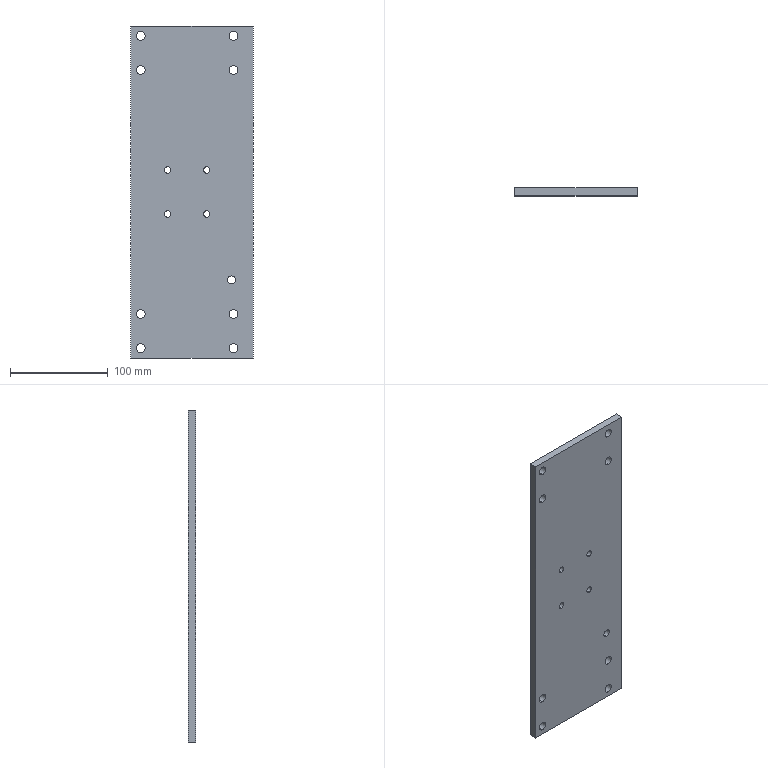Part | STEP file | X77-07101 | 1 solid | 32 faces | box 125 x 8 x 340 mm | volume 334465 mm3 | cylinder 26 | plane 6 | commonest cylinder face diameters 9 x16 6.5 x8 8 x2
STEP:
#1=CARTESIAN_POINT('',(-140.231,-59.214,-256.));
#2=VERTEX_POINT('',#1);
#3=CARTESIAN_POINT('',(-140.231,-59.214,-264.));
#4=VERTEX_POINT('',#3);
#5=CARTESIAN_POINT('',(-140.231,-59.214,-260.));
#6=DIRECTION('',(0.,-1.,0.));
#7=DIRECTION('',(1.,0.,0.));
#8=AXIS2_PLACEMENT_3D('',#5,#6,#7);
#9=CIRCLE('',#8,4.);
#10=EDGE_CURVE('',#2,#4,#9,.T.);
#11=ORIENTED_EDGE('',*,*,#10,.T.);
#12=CARTESIAN_POINT('',(-140.231,-51.214,-264.));
#13=VERTEX_POINT('',#12);
#14=CARTESIAN_POINT('',(-140.231,-51.214,-264.));
#15=DIRECTION('',(0.,1.,0.));
#16=VECTOR('',#15,1000.);
#17=LINE('',#14,#16);
#18=EDGE_CURVE('',#4,#13,#17,.T.);
#19=ORIENTED_EDGE('',*,*,#18,.T.);
#20=CARTESIAN_POINT('',(-140.231,-51.214,-256.));
#21=VERTEX_POINT('',#20);
#22=CARTESIAN_POINT('',(-140.231,-51.214,-260.));
#23=DIRECTION('',(0.,1.,0.));
#24=DIRECTION('',(0.,0.,1.));
#25=AXIS2_PLACEMENT_3D('',#22,#23,#24);
#26=CIRCLE('',#25,4.);
#27=EDGE_CURVE('',#13,#21,#26,.T.);
#28=ORIENTED_EDGE('',*,*,#27,.T.);
#29=CARTESIAN_POINT('',(-140.231,-51.214,-256.));
#30=DIRECTION('',(0.,1.,0.));
#31=VECTOR('',#30,1000.);
#32=LINE('',#29,#31);
#33=EDGE_CURVE('',#2,#21,#32,.T.);
#34=ORIENTED_EDGE('',*,*,#33,.F.);
#35=EDGE_LOOP('',(#11,#19,#28,#34));
#36=FACE_OUTER_BOUND('',#35,.T.);
#37=CARTESIAN_POINT('',(-140.231,-51.214,-260.));
#38=DIRECTION('',(0.,1.,0.));
#39=DIRECTION('',(0.,0.,1.));
#40=AXIS2_PLACEMENT_3D('',#37,#38,#39);
#41=CYLINDRICAL_SURFACE('',#40,4.);
#42=ADVANCED_FACE('',(#36),#41,.F.);
#43=CARTESIAN_POINT('',(-138.186,-51.214,-334.5));
#44=VERTEX_POINT('',#43);
#45=CARTESIAN_POINT('',(-138.186,-51.214,-325.5));
#46=VERTEX_POINT('',#45);
#47=CARTESIAN_POINT('',(-138.186,-51.214,-330.));
#48=DIRECTION('',(0.,1.,0.));
#49=DIRECTION('',(0.,0.,1.));
#50=AXIS2_PLACEMENT_3D('',#47,#48,#49);
#51=CIRCLE('',#50,4.5);
#52=EDGE_CURVE('',#44,#46,#51,.T.);
#53=ORIENTED_EDGE('',*,*,#52,.T.);
#54=CARTESIAN_POINT('',(-138.186,-59.214,-325.5));
#55=VERTEX_POINT('',#54);
#56=CARTESIAN_POINT('',(-138.186,-59.214,-325.5));
#57=DIRECTION('',(0.,-1.,0.));
#58=VECTOR('',#57,1000.);
#59=LINE('',#56,#58);
#60=EDGE_CURVE('',#46,#55,#59,.T.);
#61=ORIENTED_EDGE('',*,*,#60,.T.);
#62=CARTESIAN_POINT('',(-138.186,-59.214,-334.5));
#63=VERTEX_POINT('',#62);
#64=CARTESIAN_POINT('',(-138.186,-59.214,-330.));
#65=DIRECTION('',(0.,-1.,0.));
#66=DIRECTION('',(0.,0.,-1.));
#67=AXIS2_PLACEMENT_3D('',#64,#65,#66);
#68=CIRCLE('',#67,4.5);
#69=EDGE_CURVE('',#55,#63,#68,.T.);
#70=ORIENTED_EDGE('',*,*,#69,.T.);
#71=CARTESIAN_POINT('',(-138.186,-59.214,-334.5));
#72=DIRECTION('',(0.,-1.,0.));
#73=VECTOR('',#72,1000.);
#74=LINE('',#71,#73);
#75=EDGE_CURVE('',#44,#63,#74,.T.);
#76=ORIENTED_EDGE('',*,*,#75,.F.);
#77=EDGE_LOOP('',(#53,#61,#70,#76));
#78=FACE_OUTER_BOUND('',#77,.T.);
#79=CARTESIAN_POINT('',(-138.186,-59.214,-330.));
#80=DIRECTION('',(0.,-1.,0.));
#81=DIRECTION('',(0.,0.,-1.));
#82=AXIS2_PLACEMENT_3D('',#79,#80,#81);
#83=CYLINDRICAL_SURFACE('',#82,4.5);
#84=ADVANCED_FACE('',(#78),#83,.F.);
#85=CARTESIAN_POINT('',(-233.199,-51.214,-334.5));
#86=VERTEX_POINT('',#85);
#87=CARTESIAN_POINT('',(-233.199,-51.214,-325.5));
#88=VERTEX_POINT('',#87);
#89=CARTESIAN_POINT('',(-233.199,-51.214,-330.));
#90=DIRECTION('',(0.,1.,0.));
#91=DIRECTION('',(0.,0.,1.));
#92=AXIS2_PLACEMENT_3D('',#89,#90,#91);
#93=CIRCLE('',#92,4.5);
#94=EDGE_CURVE('',#86,#88,#93,.T.);
#95=ORIENTED_EDGE('',*,*,#94,.T.);
#96=CARTESIAN_POINT('',(-233.199,-59.214,-325.5));
#97=VERTEX_POINT('',#96);
#98=CARTESIAN_POINT('',(-233.199,-59.214,-325.5));
#99=DIRECTION('',(0.,-1.,0.));
#100=VECTOR('',#99,1000.);
#101=LINE('',#98,#100);
#102=EDGE_CURVE('',#88,#97,#101,.T.);
#103=ORIENTED_EDGE('',*,*,#102,.T.);
#104=CARTESIAN_POINT('',(-233.199,-59.214,-334.5));
#105=VERTEX_POINT('',#104);
#106=CARTESIAN_POINT('',(-233.199,-59.214,-330.));
#107=DIRECTION('',(0.,-1.,0.));
#108=DIRECTION('',(0.,0.,-1.));
#109=AXIS2_PLACEMENT_3D('',#106,#107,#108);
#110=CIRCLE('',#109,4.5);
#111=EDGE_CURVE('',#97,#105,#110,.T.);
#112=ORIENTED_EDGE('',*,*,#111,.T.);
#113=CARTESIAN_POINT('',(-233.199,-59.214,-334.5));
#114=DIRECTION('',(0.,-1.,0.));
#115=VECTOR('',#114,1000.);
#116=LINE('',#113,#115);
#117=EDGE_CURVE('',#86,#105,#116,.T.);
#118=ORIENTED_EDGE('',*,*,#117,.F.);
#119=EDGE_LOOP('',(#95,#103,#112,#118));
#120=FACE_OUTER_BOUND('',#119,.T.);
#121=CARTESIAN_POINT('',(-233.199,-59.214,-330.));
#122=DIRECTION('',(0.,-1.,0.));
#123=DIRECTION('',(0.,0.,-1.));
#124=AXIS2_PLACEMENT_3D('',#121,#122,#123);
#125=CYLINDRICAL_SURFACE('',#124,4.5);
#126=ADVANCED_FACE('',(#120),#125,.F.);
#127=CARTESIAN_POINT('',(-233.199,-51.214,-299.5));
#128=VERTEX_POINT('',#127);
#129=CARTESIAN_POINT('',(-233.199,-51.214,-290.5));
#130=VERTEX_POINT('',#129);
#131=CARTESIAN_POINT('',(-233.199,-51.214,-295.));
#132=DIRECTION('',(0.,1.,0.));
#133=DIRECTION('',(0.,0.,1.));
#134=AXIS2_PLACEMENT_3D('',#131,#132,#133);
#135=CIRCLE('',#134,4.5);
#136=EDGE_CURVE('',#128,#130,#135,.T.);
#137=ORIENTED_EDGE('',*,*,#136,.T.);
#138=CARTESIAN_POINT('',(-233.199,-59.214,-290.5));
#139=VERTEX_POINT('',#138);
#140=CARTESIAN_POINT('',(-233.199,-59.214,-290.5));
#141=DIRECTION('',(0.,-1.,0.));
#142=VECTOR('',#141,1000.);
#143=LINE('',#140,#142);
#144=EDGE_CURVE('',#130,#139,#143,.T.);
#145=ORIENTED_EDGE('',*,*,#144,.T.);
#146=CARTESIAN_POINT('',(-233.199,-59.214,-299.5));
#147=VERTEX_POINT('',#146);
#148=CARTESIAN_POINT('',(-233.199,-59.214,-295.));
#149=DIRECTION('',(0.,-1.,0.));
#150=DIRECTION('',(0.,0.,-1.));
#151=AXIS2_PLACEMENT_3D('',#148,#149,#150);
#152=CIRCLE('',#151,4.5);
#153=EDGE_CURVE('',#139,#147,#152,.T.);
#154=ORIENTED_EDGE('',*,*,#153,.T.);
#155=CARTESIAN_POINT('',(-233.199,-59.214,-299.5));
#156=DIRECTION('',(0.,-1.,0.));
#157=VECTOR('',#156,1000.);
#158=LINE('',#155,#157);
#159=EDGE_CURVE('',#128,#147,#158,.T.);
#160=ORIENTED_EDGE('',*,*,#159,.F.);
#161=EDGE_LOOP('',(#137,#145,#154,#160));
#162=FACE_OUTER_BOUND('',#161,.T.);
#163=CARTESIAN_POINT('',(-233.199,-59.214,-295.));
#164=DIRECTION('',(0.,-1.,0.));
#165=DIRECTION('',(0.,0.,-1.));
#166=AXIS2_PLACEMENT_3D('',#163,#164,#165);
#167=CYLINDRICAL_SURFACE('',#166,4.5);
#168=ADVANCED_FACE('',(#162),#167,.F.);
#169=CARTESIAN_POINT('',(-138.139,-51.214,-299.5));
#170=VERTEX_POINT('',#169);
#171=CARTESIAN_POINT('',(-138.139,-51.214,-290.5));
#172=VERTEX_POINT('',#171);
#173=CARTESIAN_POINT('',(-138.139,-51.214,-295.));
#174=DIRECTION('',(0.,1.,0.));
#175=DIRECTION('',(0.,0.,1.));
#176=AXIS2_PLACEMENT_3D('',#173,#174,#175);
#177=CIRCLE('',#176,4.5);
#178=EDGE_CURVE('',#170,#172,#177,.T.);
#179=ORIENTED_EDGE('',*,*,#178,.T.);
#180=CARTESIAN_POINT('',(-138.139,-59.214,-290.5));
#181=VERTEX_POINT('',#180);
#182=CARTESIAN_POINT('',(-138.139,-59.214,-290.5));
#183=DIRECTION('',(0.,-1.,0.));
#184=VECTOR('',#183,1000.);
#185=LINE('',#182,#184);
#186=EDGE_CURVE('',#172,#181,#185,.T.);
#187=ORIENTED_EDGE('',*,*,#186,.T.);
#188=CARTESIAN_POINT('',(-138.139,-59.214,-299.5));
#189=VERTEX_POINT('',#188);
#190=CARTESIAN_POINT('',(-138.139,-59.214,-295.));
#191=DIRECTION('',(0.,-1.,0.));
#192=DIRECTION('',(0.,0.,-1.));
#193=AXIS2_PLACEMENT_3D('',#190,#191,#192);
#194=CIRCLE('',#193,4.5);
#195=EDGE_CURVE('',#181,#189,#194,.T.);
#196=ORIENTED_EDGE('',*,*,#195,.T.);
#197=CARTESIAN_POINT('',(-138.139,-59.214,-299.5));
#198=DIRECTION('',(0.,-1.,0.));
#199=VECTOR('',#198,1000.);
#200=LINE('',#197,#199);
#201=EDGE_CURVE('',#170,#189,#200,.T.);
#202=ORIENTED_EDGE('',*,*,#201,.F.);
#203=EDGE_LOOP('',(#179,#187,#196,#202));
#204=FACE_OUTER_BOUND('',#203,.T.);
#205=CARTESIAN_POINT('',(-138.139,-59.214,-295.));
#206=DIRECTION('',(0.,-1.,0.));
#207=DIRECTION('',(0.,0.,-1.));
#208=AXIS2_PLACEMENT_3D('',#205,#206,#207);
#209=CYLINDRICAL_SURFACE('',#208,4.5);
#210=ADVANCED_FACE('',(#204),#209,.F.);
#211=CARTESIAN_POINT('',(-233.199,-51.214,-14.5));
#212=VERTEX_POINT('',#211);
#213=CARTESIAN_POINT('',(-233.199,-51.214,-5.5));
#214=VERTEX_POINT('',#213);
#215=CARTESIAN_POINT('',(-233.199,-51.214,-10.));
#216=DIRECTION('',(0.,1.,0.));
#217=DIRECTION('',(0.,0.,1.));
#218=AXIS2_PLACEMENT_3D('',#215,#216,#217);
#219=CIRCLE('',#218,4.5);
#220=EDGE_CURVE('',#212,#214,#219,.T.);
#221=ORIENTED_EDGE('',*,*,#220,.T.);
#222=CARTESIAN_POINT('',(-233.199,-59.214,-5.5));
#223=VERTEX_POINT('',#222);
#224=CARTESIAN_POINT('',(-233.199,-59.214,-5.5));
#225=DIRECTION('',(0.,-1.,0.));
#226=VECTOR('',#225,1000.);
#227=LINE('',#224,#226);
#228=EDGE_CURVE('',#214,#223,#227,.T.);
#229=ORIENTED_EDGE('',*,*,#228,.T.);
#230=CARTESIAN_POINT('',(-233.199,-59.214,-14.5));
#231=VERTEX_POINT('',#230);
#232=CARTESIAN_POINT('',(-233.199,-59.214,-10.));
#233=DIRECTION('',(0.,-1.,0.));
#234=DIRECTION('',(0.,0.,-1.));
#235=AXIS2_PLACEMENT_3D('',#232,#233,#234);
#236=CIRCLE('',#235,4.5);
#237=EDGE_CURVE('',#223,#231,#236,.T.);
#238=ORIENTED_EDGE('',*,*,#237,.T.);
#239=CARTESIAN_POINT('',(-233.199,-59.214,-14.5));
#240=DIRECTION('',(0.,-1.,0.));
#241=VECTOR('',#240,1000.);
#242=LINE('',#239,#241);
#243=EDGE_CURVE('',#212,#231,#242,.T.);
#244=ORIENTED_EDGE('',*,*,#243,.F.);
#245=EDGE_LOOP('',(#221,#229,#238,#244));
#246=FACE_OUTER_BOUND('',#245,.T.);
#247=CARTESIAN_POINT('',(-233.199,-59.214,-10.));
#248=DIRECTION('',(0.,-1.,0.));
#249=DIRECTION('',(0.,0.,-1.));
#250=AXIS2_PLACEMENT_3D('',#247,#248,#249);
#251=CYLINDRICAL_SURFACE('',#250,4.5);
#252=ADVANCED_FACE('',(#246),#251,.F.);
#253=CARTESIAN_POINT('',(-138.186,-51.214,-14.5));
#254=VERTEX_POINT('',#253);
#255=CARTESIAN_POINT('',(-138.186,-51.214,-5.5));
#256=VERTEX_POINT('',#255);
#257=CARTESIAN_POINT('',(-138.186,-51.214,-10.));
#258=DIRECTION('',(0.,1.,0.));
#259=DIRECTION('',(0.,0.,1.));
#260=AXIS2_PLACEMENT_3D('',#257,#258,#259);
#261=CIRCLE('',#260,4.5);
#262=EDGE_CURVE('',#254,#256,#261,.T.);
#263=ORIENTED_EDGE('',*,*,#262,.T.);
#264=CARTESIAN_POINT('',(-138.186,-59.214,-5.5));
#265=VERTEX_POINT('',#264);
#266=CARTESIAN_POINT('',(-138.186,-59.214,-5.5));
#267=DIRECTION('',(0.,-1.,0.));
#268=VECTOR('',#267,1000.);
#269=LINE('',#266,#268);
#270=EDGE_CURVE('',#256,#265,#269,.T.);
#271=ORIENTED_EDGE('',*,*,#270,.T.);
#272=CARTESIAN_POINT('',(-138.186,-59.214,-14.5));
#273=VERTEX_POINT('',#272);
#274=CARTESIAN_POINT('',(-138.186,-59.214,-10.));
#275=DIRECTION('',(0.,-1.,0.));
#276=DIRECTION('',(0.,0.,-1.));
#277=AXIS2_PLACEMENT_3D('',#274,#275,#276);
#278=CIRCLE('',#277,4.5);
#279=EDGE_CURVE('',#265,#273,#278,.T.);
#280=ORIENTED_EDGE('',*,*,#279,.T.);
#281=CARTESIAN_POINT('',(-138.186,-59.214,-14.5));
#282=DIRECTION('',(0.,-1.,0.));
#283=VECTOR('',#282,1000.);
#284=LINE('',#281,#283);
#285=EDGE_CURVE('',#254,#273,#284,.T.);
#286=ORIENTED_EDGE('',*,*,#285,.F.);
#287=EDGE_LOOP('',(#263,#271,#280,#286));
#288=FACE_OUTER_BOUND('',#287,.T.);
#289=CARTESIAN_POINT('',(-138.186,-59.214,-10.));
#290=DIRECTION('',(0.,-1.,0.));
#291=DIRECTION('',(0.,0.,-1.));
#292=AXIS2_PLACEMENT_3D('',#289,#290,#291);
#293=CYLINDRICAL_SURFACE('',#292,4.5);
#294=ADVANCED_FACE('',(#288),#293,.F.);
#295=CARTESIAN_POINT('',(-138.139,-51.214,-49.5));
#296=VERTEX_POINT('',#295);
#297=CARTESIAN_POINT('',(-138.139,-51.214,-40.5));
#298=VERTEX_POINT('',#297);
#299=CARTESIAN_POINT('',(-138.139,-51.214,-45.));
#300=DIRECTION('',(0.,1.,0.));
#301=DIRECTION('',(0.,0.,1.));
#302=AXIS2_PLACEMENT_3D('',#299,#300,#301);
#303=CIRCLE('',#302,4.5);
#304=EDGE_CURVE('',#296,#298,#303,.T.);
#305=ORIENTED_EDGE('',*,*,#304,.T.);
#306=CARTESIAN_POINT('',(-138.139,-59.214,-40.5));
#307=VERTEX_POINT('',#306);
#308=CARTESIAN_POINT('',(-138.139,-59.214,-40.5));
#309=DIRECTION('',(0.,-1.,0.));
#310=VECTOR('',#309,1000.);
#311=LINE('',#308,#310);
#312=EDGE_CURVE('',#298,#307,#311,.T.);
#313=ORIENTED_EDGE('',*,*,#312,.T.);
#314=CARTESIAN_POINT('',(-138.139,-59.214,-49.5));
#315=VERTEX_POINT('',#314);
#316=CARTESIAN_POINT('',(-138.139,-59.214,-45.));
#317=DIRECTION('',(0.,-1.,0.));
#318=DIRECTION('',(0.,0.,-1.));
#319=AXIS2_PLACEMENT_3D('',#316,#317,#318);
#320=CIRCLE('',#319,4.5);
#321=EDGE_CURVE('',#307,#315,#320,.T.);
#322=ORIENTED_EDGE('',*,*,#321,.T.);
#323=CARTESIAN_POINT('',(-138.139,-59.214,-49.5));
#324=DIRECTION('',(0.,-1.,0.));
#325=VECTOR('',#324,1000.);
#326=LINE('',#323,#325);
#327=EDGE_CURVE('',#296,#315,#326,.T.);
#328=ORIENTED_EDGE('',*,*,#327,.F.);
#329=EDGE_LOOP('',(#305,#313,#322,#328));
#330=FACE_OUTER_BOUND('',#329,.T.);
#331=CARTESIAN_POINT('',(-138.139,-59.214,-45.));
#332=DIRECTION('',(0.,-1.,0.));
#333=DIRECTION('',(0.,0.,-1.));
#334=AXIS2_PLACEMENT_3D('',#331,#332,#333);
#335=CYLINDRICAL_SURFACE('',#334,4.5);
#336=ADVANCED_FACE('',(#330),#335,.F.);
#337=CARTESIAN_POINT('',(-233.199,-51.214,-49.5));
#338=VERTEX_POINT('',#337);
#339=CARTESIAN_POINT('',(-233.199,-51.214,-40.5));
#340=VERTEX_POINT('',#339);
#341=CARTESIAN_POINT('',(-233.199,-51.214,-45.));
#342=DIRECTION('',(0.,1.,0.));
#343=DIRECTION('',(0.,0.,1.));
#344=AXIS2_PLACEMENT_3D('',#341,#342,#343);
#345=CIRCLE('',#344,4.5);
#346=EDGE_CURVE('',#338,#340,#345,.T.);
#347=ORIENTED_EDGE('',*,*,#346,.T.);
#348=CARTESIAN_POINT('',(-233.199,-59.214,-40.5));
#349=VERTEX_POINT('',#348);
#350=CARTESIAN_POINT('',(-233.199,-59.214,-40.5));
#351=DIRECTION('',(0.,-1.,0.));
#352=VECTOR('',#351,1000.);
#353=LINE('',#350,#352);
#354=EDGE_CURVE('',#340,#349,#353,.T.);
#355=ORIENTED_EDGE('',*,*,#354,.T.);
#356=CARTESIAN_POINT('',(-233.199,-59.214,-49.5));
#357=VERTEX_POINT('',#356);
#358=CARTESIAN_POINT('',(-233.199,-59.214,-45.));
#359=DIRECTION('',(0.,-1.,0.));
#360=DIRECTION('',(0.,0.,-1.));
#361=AXIS2_PLACEMENT_3D('',#358,#359,#360);
#362=CIRCLE('',#361,4.5);
#363=EDGE_CURVE('',#349,#357,#362,.T.);
#364=ORIENTED_EDGE('',*,*,#363,.T.);
#365=CARTESIAN_POINT('',(-233.199,-59.214,-49.5));
#366=DIRECTION('',(0.,-1.,0.));
#367=VECTOR('',#366,1000.);
#368=LINE('',#365,#367);
#369=EDGE_CURVE('',#338,#357,#368,.T.);
#370=ORIENTED_EDGE('',*,*,#369,.F.);
#371=EDGE_LOOP('',(#347,#355,#364,#370));
#372=FACE_OUTER_BOUND('',#371,.T.);
#373=CARTESIAN_POINT('',(-233.199,-59.214,-45.));
#374=DIRECTION('',(0.,-1.,0.));
#375=DIRECTION('',(0.,0.,-1.));
#376=AXIS2_PLACEMENT_3D('',#373,#374,#375);
#377=CYLINDRICAL_SURFACE('',#376,4.5);
#378=ADVANCED_FACE('',(#372),#377,.F.);
#379=CARTESIAN_POINT('',(-205.699,-51.214,-195.75));
#380=VERTEX_POINT('',#379);
#381=CARTESIAN_POINT('',(-205.699,-51.214,-189.25));
#382=VERTEX_POINT('',#381);
#383=CARTESIAN_POINT('',(-205.699,-51.214,-192.5));
#384=DIRECTION('',(0.,1.,0.));
#385=DIRECTION('',(0.,0.,1.));
#386=AXIS2_PLACEMENT_3D('',#383,#384,#385);
#387=CIRCLE('',#386,3.25);
#388=EDGE_CURVE('',#380,#382,#387,.T.);
#389=ORIENTED_EDGE('',*,*,#388,.T.);
#390=CARTESIAN_POINT('',(-205.699,-59.214,-189.25));
#391=VERTEX_POINT('',#390);
#392=CARTESIAN_POINT('',(-205.699,-59.214,-189.25));
#393=DIRECTION('',(0.,-1.,0.));
#394=VECTOR('',#393,1000.);
#395=LINE('',#392,#394);
#396=EDGE_CURVE('',#382,#391,#395,.T.);
#397=ORIENTED_EDGE('',*,*,#396,.T.);
#398=CARTESIAN_POINT('',(-205.699,-59.214,-195.75));
#399=VERTEX_POINT('',#398);
#400=CARTESIAN_POINT('',(-205.699,-59.214,-192.5));
#401=DIRECTION('',(0.,-1.,0.));
#402=DIRECTION('',(0.,0.,-1.));
#403=AXIS2_PLACEMENT_3D('',#400,#401,#402);
#404=CIRCLE('',#403,3.25);
#405=EDGE_CURVE('',#391,#399,#404,.T.);
#406=ORIENTED_EDGE('',*,*,#405,.T.);
#407=CARTESIAN_POINT('',(-205.699,-59.214,-195.75));
#408=DIRECTION('',(0.,-1.,0.));
#409=VECTOR('',#408,1000.);
#410=LINE('',#407,#409);
#411=EDGE_CURVE('',#380,#399,#410,.T.);
#412=ORIENTED_EDGE('',*,*,#411,.F.);
#413=EDGE_LOOP('',(#389,#397,#406,#412));
#414=FACE_OUTER_BOUND('',#413,.T.);
#415=CARTESIAN_POINT('',(-205.699,-59.214,-192.5));
#416=DIRECTION('',(0.,-1.,0.));
#417=DIRECTION('',(0.,0.,-1.));
#418=AXIS2_PLACEMENT_3D('',#415,#416,#417);
#419=CYLINDRICAL_SURFACE('',#418,3.25);
#420=ADVANCED_FACE('',(#414),#419,.F.);
#421=CARTESIAN_POINT('',(-205.699,-51.214,-150.75));
#422=VERTEX_POINT('',#421);
#423=CARTESIAN_POINT('',(-205.699,-51.214,-144.25));
#424=VERTEX_POINT('',#423);
#425=CARTESIAN_POINT('',(-205.699,-51.214,-147.5));
#426=DIRECTION('',(0.,1.,0.));
#427=DIRECTION('',(0.,0.,1.));
#428=AXIS2_PLACEMENT_3D('',#425,#426,#427);
#429=CIRCLE('',#428,3.25);
#430=EDGE_CURVE('',#422,#424,#429,.T.);
#431=ORIENTED_EDGE('',*,*,#430,.T.);
#432=CARTESIAN_POINT('',(-205.699,-59.214,-144.25));
#433=VERTEX_POINT('',#432);
#434=CARTESIAN_POINT('',(-205.699,-59.214,-144.25));
#435=DIRECTION('',(0.,-1.,0.));
#436=VECTOR('',#435,1000.);
#437=LINE('',#434,#436);
#438=EDGE_CURVE('',#424,#433,#437,.T.);
#439=ORIENTED_EDGE('',*,*,#438,.T.);
#440=CARTESIAN_POINT('',(-205.699,-59.214,-150.75));
#441=VERTEX_POINT('',#440);
#442=CARTESIAN_POINT('',(-205.699,-59.214,-147.5));
#443=DIRECTION('',(0.,-1.,0.));
#444=DIRECTION('',(0.,0.,-1.));
#445=AXIS2_PLACEMENT_3D('',#442,#443,#444);
#446=CIRCLE('',#445,3.25);
#447=EDGE_CURVE('',#433,#441,#446,.T.);
#448=ORIENTED_EDGE('',*,*,#447,.T.);
#449=CARTESIAN_POINT('',(-205.699,-59.214,-150.75));
#450=DIRECTION('',(0.,-1.,0.));
#451=VECTOR('',#450,1000.);
#452=LINE('',#449,#451);
#453=EDGE_CURVE('',#422,#441,#452,.T.);
#454=ORIENTED_EDGE('',*,*,#453,.F.);
#455=EDGE_LOOP('',(#431,#439,#448,#454));
#456=FACE_OUTER_BOUND('',#455,.T.);
#457=CARTESIAN_POINT('',(-205.699,-59.214,-147.5));
#458=DIRECTION('',(0.,-1.,0.));
#459=DIRECTION('',(0.,0.,-1.));
#460=AXIS2_PLACEMENT_3D('',#457,#458,#459);
#461=CYLINDRICAL_SURFACE('',#460,3.25);
#462=ADVANCED_FACE('',(#456),#461,.F.);
#463=CARTESIAN_POINT('',(-165.699,-51.214,-195.75));
#464=VERTEX_POINT('',#463);
#465=CARTESIAN_POINT('',(-165.699,-51.214,-189.25));
#466=VERTEX_POINT('',#465);
#467=CARTESIAN_POINT('',(-165.699,-51.214,-192.5));
#468=DIRECTION('',(0.,1.,0.));
#469=DIRECTION('',(0.,0.,1.));
#470=AXIS2_PLACEMENT_3D('',#467,#468,#469);
#471=CIRCLE('',#470,3.25);
#472=EDGE_CURVE('',#464,#466,#471,.T.);
#473=ORIENTED_EDGE('',*,*,#472,.T.);
#474=CARTESIAN_POINT('',(-165.699,-59.214,-189.25));
#475=VERTEX_POINT('',#474);
#476=CARTESIAN_POINT('',(-165.699,-59.214,-189.25));
#477=DIRECTION('',(0.,-1.,0.));
#478=VECTOR('',#477,1000.);
#479=LINE('',#476,#478);
#480=EDGE_CURVE('',#466,#475,#479,.T.);
#481=ORIENTED_EDGE('',*,*,#480,.T.);
#482=CARTESIAN_POINT('',(-165.699,-59.214,-195.75));
#483=VERTEX_POINT('',#482);
#484=CARTESIAN_POINT('',(-165.699,-59.214,-192.5));
#485=DIRECTION('',(0.,-1.,0.));
#486=DIRECTION('',(0.,0.,-1.));
#487=AXIS2_PLACEMENT_3D('',#484,#485,#486);
#488=CIRCLE('',#487,3.25);
#489=EDGE_CURVE('',#475,#483,#488,.T.);
#490=ORIENTED_EDGE('',*,*,#489,.T.);
#491=CARTESIAN_POINT('',(-165.699,-59.214,-195.75));
#492=DIRECTION('',(0.,-1.,0.));
#493=VECTOR('',#492,1000.);
#494=LINE('',#491,#493);
#495=EDGE_CURVE('',#464,#483,#494,.T.);
#496=ORIENTED_EDGE('',*,*,#495,.F.);
#497=EDGE_LOOP('',(#473,#481,#490,#496));
#498=FACE_OUTER_BOUND('',#497,.T.);
#499=CARTESIAN_POINT('',(-165.699,-59.214,-192.5));
#500=DIRECTION('',(0.,-1.,0.));
#501=DIRECTION('',(0.,0.,-1.));
#502=AXIS2_PLACEMENT_3D('',#499,#500,#501);
#503=CYLINDRICAL_SURFACE('',#502,3.25);
#504=ADVANCED_FACE('',(#498),#503,.F.);
#505=CARTESIAN_POINT('',(-165.699,-51.214,-150.75));
#506=VERTEX_POINT('',#505);
#507=CARTESIAN_POINT('',(-165.699,-51.214,-144.25));
#508=VERTEX_POINT('',#507);
#509=CARTESIAN_POINT('',(-165.699,-51.214,-147.5));
#510=DIRECTION('',(0.,1.,0.));
#511=DIRECTION('',(0.,0.,1.));
#512=AXIS2_PLACEMENT_3D('',#509,#510,#511);
#513=CIRCLE('',#512,3.25);
#514=EDGE_CURVE('',#506,#508,#513,.T.);
#515=ORIENTED_EDGE('',*,*,#514,.T.);
#516=CARTESIAN_POINT('',(-165.699,-59.214,-144.25));
#517=VERTEX_POINT('',#516);
#518=CARTESIAN_POINT('',(-165.699,-59.214,-144.25));
#519=DIRECTION('',(0.,-1.,0.));
#520=VECTOR('',#519,1000.);
#521=LINE('',#518,#520);
#522=EDGE_CURVE('',#508,#517,#521,.T.);
#523=ORIENTED_EDGE('',*,*,#522,.T.);
#524=CARTESIAN_POINT('',(-165.699,-59.214,-150.75));
#525=VERTEX_POINT('',#524);
#526=CARTESIAN_POINT('',(-165.699,-59.214,-147.5));
#527=DIRECTION('',(0.,-1.,0.));
#528=DIRECTION('',(0.,0.,-1.));
#529=AXIS2_PLACEMENT_3D('',#526,#527,#528);
#530=CIRCLE('',#529,3.25);
#531=EDGE_CURVE('',#517,#525,#530,.T.);
#532=ORIENTED_EDGE('',*,*,#531,.T.);
#533=CARTESIAN_POINT('',(-165.699,-59.214,-150.75));
#534=DIRECTION('',(0.,-1.,0.));
#535=VECTOR('',#534,1000.);
#536=LINE('',#533,#535);
#537=EDGE_CURVE('',#506,#525,#536,.T.);
#538=ORIENTED_EDGE('',*,*,#537,.F.);
#539=EDGE_LOOP('',(#515,#523,#532,#538));
#540=FACE_OUTER_BOUND('',#539,.T.);
#541=CARTESIAN_POINT('',(-165.699,-59.214,-147.5));
#542=DIRECTION('',(0.,-1.,0.));
#543=DIRECTION('',(0.,0.,-1.));
#544=AXIS2_PLACEMENT_3D('',#541,#542,#543);
#545=CYLINDRICAL_SURFACE('',#544,3.25);
#546=ADVANCED_FACE('',(#540),#545,.F.);
#547=CARTESIAN_POINT('',(-243.199,-51.214,0.));
#548=VERTEX_POINT('',#547);
#549=CARTESIAN_POINT('',(-243.199,-59.214,0.));
#550=VERTEX_POINT('',#549);
#551=CARTESIAN_POINT('',(-243.199,-51.214,0.));
#552=DIRECTION('',(0.,-1.,0.));
#553=VECTOR('',#552,1000.);
#554=LINE('',#551,#553);
#555=EDGE_CURVE('',#548,#550,#554,.T.);
#556=ORIENTED_EDGE('',*,*,#555,.F.);
#557=CARTESIAN_POINT('',(-243.199,-51.214,-340.));
#558=VERTEX_POINT('',#557);
#559=CARTESIAN_POINT('',(-243.199,-51.214,-340.));
#560=DIRECTION('',(0.,0.,1.));
#561=VECTOR('',#560,1000.);
#562=LINE('',#559,#561);
#563=EDGE_CURVE('',#558,#548,#562,.T.);
#564=ORIENTED_EDGE('',*,*,#563,.F.);
#565=CARTESIAN_POINT('',(-243.199,-59.214,-340.));
#566=VERTEX_POINT('',#565);
#567=CARTESIAN_POINT('',(-243.199,-51.214,-340.));
#568=DIRECTION('',(0.,-1.,0.));
#569=VECTOR('',#568,1000.);
#570=LINE('',#567,#569);
#571=EDGE_CURVE('',#558,#566,#570,.T.);
#572=ORIENTED_EDGE('',*,*,#571,.T.);
#573=CARTESIAN_POINT('',(-243.199,-59.214,-340.));
#574=DIRECTION('',(0.,0.,1.));
#575=VECTOR('',#574,1000.);
#576=LINE('',#573,#575);
#577=EDGE_CURVE('',#566,#550,#576,.T.);
#578=ORIENTED_EDGE('',*,*,#577,.T.);
#579=EDGE_LOOP('',(#556,#564,#572,#578));
#580=FACE_OUTER_BOUND('',#579,.T.);
#581=CARTESIAN_POINT('',(-243.199,-51.214,-340.));
#582=DIRECTION('',(-1.,0.,0.));
#583=DIRECTION('',(0.,0.,1.));
#584=AXIS2_PLACEMENT_3D('',#581,#582,#583);
#585=PLANE('',#584);
#586=ADVANCED_FACE('',(#580),#585,.T.);
#587=CARTESIAN_POINT('',(-140.231,-51.214,-260.));
#588=DIRECTION('',(0.,1.,0.));
#589=DIRECTION('',(0.,0.,1.));
#590=AXIS2_PLACEMENT_3D('',#587,#588,#589);
#591=CIRCLE('',#590,4.);
#592=EDGE_CURVE('',#21,#13,#591,.T.);
#593=ORIENTED_EDGE('',*,*,#592,.F.);
#594=ORIENTED_EDGE('',*,*,#27,.F.);
#595=EDGE_LOOP('',(#593,#594));
#596=FACE_BOUND('',#595,.T.);
#597=ORIENTED_EDGE('',*,*,#52,.F.);
#598=CARTESIAN_POINT('',(-138.186,-51.214,-330.));
#599=DIRECTION('',(0.,1.,0.));
#600=DIRECTION('',(0.,0.,1.));
#601=AXIS2_PLACEMENT_3D('',#598,#599,#600);
#602=CIRCLE('',#601,4.5);
#603=EDGE_CURVE('',#46,#44,#602,.T.);
#604=ORIENTED_EDGE('',*,*,#603,.F.);
#605=EDGE_LOOP('',(#597,#604));
#606=FACE_BOUND('',#605,.T.);
#607=ORIENTED_EDGE('',*,*,#94,.F.);
#608=CARTESIAN_POINT('',(-233.199,-51.214,-330.));
#609=DIRECTION('',(0.,1.,0.));
#610=DIRECTION('',(0.,0.,1.));
#611=AXIS2_PLACEMENT_3D('',#608,#609,#610);
#612=CIRCLE('',#611,4.5);
#613=EDGE_CURVE('',#88,#86,#612,.T.);
#614=ORIENTED_EDGE('',*,*,#613,.F.);
#615=EDGE_LOOP('',(#607,#614));
#616=FACE_BOUND('',#615,.T.);
#617=ORIENTED_EDGE('',*,*,#136,.F.);
#618=CARTESIAN_POINT('',(-233.199,-51.214,-295.));
#619=DIRECTION('',(0.,1.,0.));
#620=DIRECTION('',(0.,0.,1.));
#621=AXIS2_PLACEMENT_3D('',#618,#619,#620);
#622=CIRCLE('',#621,4.5);
#623=EDGE_CURVE('',#130,#128,#622,.T.);
#624=ORIENTED_EDGE('',*,*,#623,.F.);
#625=EDGE_LOOP('',(#617,#624));
#626=FACE_BOUND('',#625,.T.);
#627=ORIENTED_EDGE('',*,*,#178,.F.);
#628=CARTESIAN_POINT('',(-138.139,-51.214,-295.));
#629=DIRECTION('',(0.,1.,0.));
#630=DIRECTION('',(0.,0.,1.));
#631=AXIS2_PLACEMENT_3D('',#628,#629,#630);
#632=CIRCLE('',#631,4.5);
#633=EDGE_CURVE('',#172,#170,#632,.T.);
#634=ORIENTED_EDGE('',*,*,#633,.F.);
#635=EDGE_LOOP('',(#627,#634));
#636=FACE_BOUND('',#635,.T.);
#637=ORIENTED_EDGE('',*,*,#220,.F.);
#638=CARTESIAN_POINT('',(-233.199,-51.214,-10.));
#639=DIRECTION('',(0.,1.,0.));
#640=DIRECTION('',(0.,0.,1.));
#641=AXIS2_PLACEMENT_3D('',#638,#639,#640);
#642=CIRCLE('',#641,4.5);
#643=EDGE_CURVE('',#214,#212,#642,.T.);
#644=ORIENTED_EDGE('',*,*,#643,.F.);
#645=EDGE_LOOP('',(#637,#644));
#646=FACE_BOUND('',#645,.T.);
#647=ORIENTED_EDGE('',*,*,#262,.F.);
#648=CARTESIAN_POINT('',(-138.186,-51.214,-10.));
#649=DIRECTION('',(0.,1.,0.));
#650=DIRECTION('',(0.,0.,1.));
#651=AXIS2_PLACEMENT_3D('',#648,#649,#650);
#652=CIRCLE('',#651,4.5);
#653=EDGE_CURVE('',#256,#254,#652,.T.);
#654=ORIENTED_EDGE('',*,*,#653,.F.);
#655=EDGE_LOOP('',(#647,#654));
#656=FACE_BOUND('',#655,.T.);
#657=ORIENTED_EDGE('',*,*,#304,.F.);
#658=CARTESIAN_POINT('',(-138.139,-51.214,-45.));
#659=DIRECTION('',(0.,1.,0.));
#660=DIRECTION('',(0.,0.,1.));
#661=AXIS2_PLACEMENT_3D('',#658,#659,#660);
#662=CIRCLE('',#661,4.5);
#663=EDGE_CURVE('',#298,#296,#662,.T.);
#664=ORIENTED_EDGE('',*,*,#663,.F.);
#665=EDGE_LOOP('',(#657,#664));
#666=FACE_BOUND('',#665,.T.);
#667=ORIENTED_EDGE('',*,*,#346,.F.);
#668=CARTESIAN_POINT('',(-233.199,-51.214,-45.));
#669=DIRECTION('',(0.,1.,0.));
#670=DIRECTION('',(0.,0.,1.));
#671=AXIS2_PLACEMENT_3D('',#668,#669,#670);
#672=CIRCLE('',#671,4.5);
#673=EDGE_CURVE('',#340,#338,#672,.T.);
#674=ORIENTED_EDGE('',*,*,#673,.F.);
#675=EDGE_LOOP('',(#667,#674));
#676=FACE_BOUND('',#675,.T.);
#677=ORIENTED_EDGE('',*,*,#388,.F.);
#678=CARTESIAN_POINT('',(-205.699,-51.214,-192.5));
#679=DIRECTION('',(0.,1.,0.));
#680=DIRECTION('',(0.,0.,1.));
#681=AXIS2_PLACEMENT_3D('',#678,#679,#680);
#682=CIRCLE('',#681,3.25);
#683=EDGE_CURVE('',#382,#380,#682,.T.);
#684=ORIENTED_EDGE('',*,*,#683,.F.);
#685=EDGE_LOOP('',(#677,#684));
#686=FACE_BOUND('',#685,.T.);
#687=ORIENTED_EDGE('',*,*,#430,.F.);
#688=CARTESIAN_POINT('',(-205.699,-51.214,-147.5));
#689=DIRECTION('',(0.,1.,0.));
#690=DIRECTION('',(0.,0.,1.));
#691=AXIS2_PLACEMENT_3D('',#688,#689,#690);
#692=CIRCLE('',#691,3.25);
#693=EDGE_CURVE('',#424,#422,#692,.T.);
#694=ORIENTED_EDGE('',*,*,#693,.F.);
#695=EDGE_LOOP('',(#687,#694));
#696=FACE_BOUND('',#695,.T.);
#697=ORIENTED_EDGE('',*,*,#472,.F.);
#698=CARTESIAN_POINT('',(-165.699,-51.214,-192.5));
#699=DIRECTION('',(0.,1.,0.));
#700=DIRECTION('',(0.,0.,1.));
#701=AXIS2_PLACEMENT_3D('',#698,#699,#700);
#702=CIRCLE('',#701,3.25);
#703=EDGE_CURVE('',#466,#464,#702,.T.);
#704=ORIENTED_EDGE('',*,*,#703,.F.);
#705=EDGE_LOOP('',(#697,#704));
#706=FACE_BOUND('',#705,.T.);
#707=ORIENTED_EDGE('',*,*,#514,.F.);
#708=CARTESIAN_POINT('',(-165.699,-51.214,-147.5));
#709=DIRECTION('',(0.,1.,0.));
#710=DIRECTION('',(0.,0.,1.));
#711=AXIS2_PLACEMENT_3D('',#708,#709,#710);
#712=CIRCLE('',#711,3.25);
#713=EDGE_CURVE('',#508,#506,#712,.T.);
#714=ORIENTED_EDGE('',*,*,#713,.F.);
#715=EDGE_LOOP('',(#707,#714));
#716=FACE_BOUND('',#715,.T.);
#717=CARTESIAN_POINT('',(-118.199,-51.214,0.));
#718=VERTEX_POINT('',#717);
#719=CARTESIAN_POINT('',(-243.199,-51.214,0.));
#720=DIRECTION('',(-1.,0.,0.));
#721=VECTOR('',#720,1000.);
#722=LINE('',#719,#721);
#723=EDGE_CURVE('',#718,#548,#722,.T.);
#724=ORIENTED_EDGE('',*,*,#723,.F.);
#725=CARTESIAN_POINT('',(-118.199,-51.214,-340.));
#726=VERTEX_POINT('',#725);
#727=CARTESIAN_POINT('',(-118.199,-51.214,-340.));
#728=DIRECTION('',(0.,0.,1.));
#729=VECTOR('',#728,1000.);
#730=LINE('',#727,#729);
#731=EDGE_CURVE('',#726,#718,#730,.T.);
#732=ORIENTED_EDGE('',*,*,#731,.F.);
#733=CARTESIAN_POINT('',(-243.199,-51.214,-340.));
#734=DIRECTION('',(-1.,0.,0.));
#735=VECTOR('',#734,1000.);
#736=LINE('',#733,#735);
#737=EDGE_CURVE('',#726,#558,#736,.T.);
#738=ORIENTED_EDGE('',*,*,#737,.T.);
#739=ORIENTED_EDGE('',*,*,#563,.T.);
#740=EDGE_LOOP('',(#724,#732,#738,#739));
#741=FACE_OUTER_BOUND('',#740,.T.);
#742=CARTESIAN_POINT('',(-243.199,-51.214,-340.));
#743=DIRECTION('',(0.,1.,0.));
#744=DIRECTION('',(0.,0.,1.));
#745=AXIS2_PLACEMENT_3D('',#742,#743,#744);
#746=PLANE('',#745);
#747=ADVANCED_FACE('',(#596,#606,#616,#626,#636,#646,#656,#666,#676,#686,#696,#706,#716,#741),#746,.T.);
#748=CARTESIAN_POINT('',(-118.199,-59.214,0.));
#749=VERTEX_POINT('',#748);
#750=CARTESIAN_POINT('',(-118.199,-51.214,0.));
#751=DIRECTION('',(0.,1.,0.));
#752=VECTOR('',#751,1000.);
#753=LINE('',#750,#752);
#754=EDGE_CURVE('',#749,#718,#753,.T.);
#755=ORIENTED_EDGE('',*,*,#754,.F.);
#756=CARTESIAN_POINT('',(-118.199,-59.214,-340.));
#757=VERTEX_POINT('',#756);
#758=CARTESIAN_POINT('',(-118.199,-59.214,-340.));
#759=DIRECTION('',(0.,0.,1.));
#760=VECTOR('',#759,1000.);
#761=LINE('',#758,#760);
#762=EDGE_CURVE('',#757,#749,#761,.T.);
#763=ORIENTED_EDGE('',*,*,#762,.F.);
#764=CARTESIAN_POINT('',(-118.199,-51.214,-340.));
#765=DIRECTION('',(0.,1.,0.));
#766=VECTOR('',#765,1000.);
#767=LINE('',#764,#766);
#768=EDGE_CURVE('',#757,#726,#767,.T.);
#769=ORIENTED_EDGE('',*,*,#768,.T.);
#770=ORIENTED_EDGE('',*,*,#731,.T.);
#771=EDGE_LOOP('',(#755,#763,#769,#770));
#772=FACE_OUTER_BOUND('',#771,.T.);
#773=CARTESIAN_POINT('',(-118.199,-51.214,-340.));
#774=DIRECTION('',(1.,0.,0.));
#775=DIRECTION('',(0.,0.,-1.));
#776=AXIS2_PLACEMENT_3D('',#773,#774,#775);
#777=PLANE('',#776);
#778=ADVANCED_FACE('',(#772),#777,.T.);
#779=ORIENTED_EDGE('',*,*,#10,.F.);
#780=CARTESIAN_POINT('',(-140.231,-59.214,-260.));
#781=DIRECTION('',(0.,-1.,0.));
#782=DIRECTION('',(1.,0.,0.));
#783=AXIS2_PLACEMENT_3D('',#780,#781,#782);
#784=CIRCLE('',#783,4.);
#785=EDGE_CURVE('',#4,#2,#784,.T.);
#786=ORIENTED_EDGE('',*,*,#785,.F.);
#787=EDGE_LOOP('',(#779,#786));
#788=FACE_BOUND('',#787,.T.);
#789=CARTESIAN_POINT('',(-138.186,-59.214,-330.));
#790=DIRECTION('',(0.,-1.,0.));
#791=DIRECTION('',(0.,0.,-1.));
#792=AXIS2_PLACEMENT_3D('',#789,#790,#791);
#793=CIRCLE('',#792,4.5);
#794=EDGE_CURVE('',#63,#55,#793,.T.);
#795=ORIENTED_EDGE('',*,*,#794,.F.);
#796=ORIENTED_EDGE('',*,*,#69,.F.);
#797=EDGE_LOOP('',(#795,#796));
#798=FACE_BOUND('',#797,.T.);
#799=CARTESIAN_POINT('',(-233.199,-59.214,-330.));
#800=DIRECTION('',(0.,-1.,0.));
#801=DIRECTION('',(0.,0.,-1.));
#802=AXIS2_PLACEMENT_3D('',#799,#800,#801);
#803=CIRCLE('',#802,4.5);
#804=EDGE_CURVE('',#105,#97,#803,.T.);
#805=ORIENTED_EDGE('',*,*,#804,.F.);
#806=ORIENTED_EDGE('',*,*,#111,.F.);
#807=EDGE_LOOP('',(#805,#806));
#808=FACE_BOUND('',#807,.T.);
#809=CARTESIAN_POINT('',(-233.199,-59.214,-295.));
#810=DIRECTION('',(0.,-1.,0.));
#811=DIRECTION('',(0.,0.,-1.));
#812=AXIS2_PLACEMENT_3D('',#809,#810,#811);
#813=CIRCLE('',#812,4.5);
#814=EDGE_CURVE('',#147,#139,#813,.T.);
#815=ORIENTED_EDGE('',*,*,#814,.F.);
#816=ORIENTED_EDGE('',*,*,#153,.F.);
#817=EDGE_LOOP('',(#815,#816));
#818=FACE_BOUND('',#817,.T.);
#819=CARTESIAN_POINT('',(-138.139,-59.214,-295.));
#820=DIRECTION('',(0.,-1.,0.));
#821=DIRECTION('',(0.,0.,-1.));
#822=AXIS2_PLACEMENT_3D('',#819,#820,#821);
#823=CIRCLE('',#822,4.5);
#824=EDGE_CURVE('',#189,#181,#823,.T.);
#825=ORIENTED_EDGE('',*,*,#824,.F.);
#826=ORIENTED_EDGE('',*,*,#195,.F.);
#827=EDGE_LOOP('',(#825,#826));
#828=FACE_BOUND('',#827,.T.);
#829=CARTESIAN_POINT('',(-233.199,-59.214,-10.));
#830=DIRECTION('',(0.,-1.,0.));
#831=DIRECTION('',(0.,0.,-1.));
#832=AXIS2_PLACEMENT_3D('',#829,#830,#831);
#833=CIRCLE('',#832,4.5);
#834=EDGE_CURVE('',#231,#223,#833,.T.);
#835=ORIENTED_EDGE('',*,*,#834,.F.);
#836=ORIENTED_EDGE('',*,*,#237,.F.);
#837=EDGE_LOOP('',(#835,#836));
#838=FACE_BOUND('',#837,.T.);
#839=CARTESIAN_POINT('',(-138.186,-59.214,-10.));
#840=DIRECTION('',(0.,-1.,0.));
#841=DIRECTION('',(0.,0.,-1.));
#842=AXIS2_PLACEMENT_3D('',#839,#840,#841);
#843=CIRCLE('',#842,4.5);
#844=EDGE_CURVE('',#273,#265,#843,.T.);
#845=ORIENTED_EDGE('',*,*,#844,.F.);
#846=ORIENTED_EDGE('',*,*,#279,.F.);
#847=EDGE_LOOP('',(#845,#846));
#848=FACE_BOUND('',#847,.T.);
#849=CARTESIAN_POINT('',(-138.139,-59.214,-45.));
#850=DIRECTION('',(0.,-1.,0.));
#851=DIRECTION('',(0.,0.,-1.));
#852=AXIS2_PLACEMENT_3D('',#849,#850,#851);
#853=CIRCLE('',#852,4.5);
#854=EDGE_CURVE('',#315,#307,#853,.T.);
#855=ORIENTED_EDGE('',*,*,#854,.F.);
#856=ORIENTED_EDGE('',*,*,#321,.F.);
#857=EDGE_LOOP('',(#855,#856));
#858=FACE_BOUND('',#857,.T.);
#859=CARTESIAN_POINT('',(-233.199,-59.214,-45.));
#860=DIRECTION('',(0.,-1.,0.));
#861=DIRECTION('',(0.,0.,-1.));
#862=AXIS2_PLACEMENT_3D('',#859,#860,#861);
#863=CIRCLE('',#862,4.5);
#864=EDGE_CURVE('',#357,#349,#863,.T.);
#865=ORIENTED_EDGE('',*,*,#864,.F.);
#866=ORIENTED_EDGE('',*,*,#363,.F.);
#867=EDGE_LOOP('',(#865,#866));
#868=FACE_BOUND('',#867,.T.);
#869=CARTESIAN_POINT('',(-205.699,-59.214,-192.5));
#870=DIRECTION('',(0.,-1.,0.));
#871=DIRECTION('',(0.,0.,-1.));
#872=AXIS2_PLACEMENT_3D('',#869,#870,#871);
#873=CIRCLE('',#872,3.25);
#874=EDGE_CURVE('',#399,#391,#873,.T.);
#875=ORIENTED_EDGE('',*,*,#874,.F.);
#876=ORIENTED_EDGE('',*,*,#405,.F.);
#877=EDGE_LOOP('',(#875,#876));
#878=FACE_BOUND('',#877,.T.);
#879=CARTESIAN_POINT('',(-205.699,-59.214,-147.5));
#880=DIRECTION('',(0.,-1.,0.));
#881=DIRECTION('',(0.,0.,-1.));
#882=AXIS2_PLACEMENT_3D('',#879,#880,#881);
#883=CIRCLE('',#882,3.25);
#884=EDGE_CURVE('',#441,#433,#883,.T.);
#885=ORIENTED_EDGE('',*,*,#884,.F.);
#886=ORIENTED_EDGE('',*,*,#447,.F.);
#887=EDGE_LOOP('',(#885,#886));
#888=FACE_BOUND('',#887,.T.);
#889=CARTESIAN_POINT('',(-165.699,-59.214,-192.5));
#890=DIRECTION('',(0.,-1.,0.));
#891=DIRECTION('',(0.,0.,-1.));
#892=AXIS2_PLACEMENT_3D('',#889,#890,#891);
#893=CIRCLE('',#892,3.25);
#894=EDGE_CURVE('',#483,#475,#893,.T.);
#895=ORIENTED_EDGE('',*,*,#894,.F.);
#896=ORIENTED_EDGE('',*,*,#489,.F.);
#897=EDGE_LOOP('',(#895,#896));
#898=FACE_BOUND('',#897,.T.);
#899=CARTESIAN_POINT('',(-165.699,-59.214,-147.5));
#900=DIRECTION('',(0.,-1.,0.));
#901=DIRECTION('',(0.,0.,-1.));
#902=AXIS2_PLACEMENT_3D('',#899,#900,#901);
#903=CIRCLE('',#902,3.25);
#904=EDGE_CURVE('',#525,#517,#903,.T.);
#905=ORIENTED_EDGE('',*,*,#904,.F.);
#906=ORIENTED_EDGE('',*,*,#531,.F.);
#907=EDGE_LOOP('',(#905,#906));
#908=FACE_BOUND('',#907,.T.);
#909=CARTESIAN_POINT('',(-118.199,-59.214,0.));
#910=DIRECTION('',(1.,0.,0.));
#911=VECTOR('',#910,1000.);
#912=LINE('',#909,#911);
#913=EDGE_CURVE('',#550,#749,#912,.T.);
#914=ORIENTED_EDGE('',*,*,#913,.F.);
#915=ORIENTED_EDGE('',*,*,#577,.F.);
#916=CARTESIAN_POINT('',(-118.199,-59.214,-340.));
#917=DIRECTION('',(1.,0.,0.));
#918=VECTOR('',#917,1000.);
#919=LINE('',#916,#918);
#920=EDGE_CURVE('',#566,#757,#919,.T.);
#921=ORIENTED_EDGE('',*,*,#920,.T.);
#922=ORIENTED_EDGE('',*,*,#762,.T.);
#923=EDGE_LOOP('',(#914,#915,#921,#922));
#924=FACE_OUTER_BOUND('',#923,.T.);
#925=CARTESIAN_POINT('',(-118.199,-59.214,-340.));
#926=DIRECTION('',(0.,-1.,0.));
#927=DIRECTION('',(1.,0.,0.));
#928=AXIS2_PLACEMENT_3D('',#925,#926,#927);
#929=PLANE('',#928);
#930=ADVANCED_FACE('',(#788,#798,#808,#818,#828,#838,#848,#858,#868,#878,#888,#898,#908,#924),#929,.T.);
#931=ORIENTED_EDGE('',*,*,#571,.F.);
#932=ORIENTED_EDGE('',*,*,#737,.F.);
#933=ORIENTED_EDGE('',*,*,#768,.F.);
#934=ORIENTED_EDGE('',*,*,#920,.F.);
#935=EDGE_LOOP('',(#931,#932,#933,#934));
#936=FACE_OUTER_BOUND('',#935,.T.);
#937=CARTESIAN_POINT('',(-243.199,-59.214,-340.));
#938=DIRECTION('',(0.,0.,-1.));
#939=DIRECTION('',(-1.,0.,0.));
#940=AXIS2_PLACEMENT_3D('',#937,#938,#939);
#941=PLANE('',#940);
#942=ADVANCED_FACE('',(#936),#941,.T.);
#943=ORIENTED_EDGE('',*,*,#555,.T.);
#944=ORIENTED_EDGE('',*,*,#913,.T.);
#945=ORIENTED_EDGE('',*,*,#754,.T.);
#946=ORIENTED_EDGE('',*,*,#723,.T.);
#947=EDGE_LOOP('',(#943,#944,#945,#946));
#948=FACE_OUTER_BOUND('',#947,.T.);
#949=CARTESIAN_POINT('',(-243.199,-59.214,0.));
#950=DIRECTION('',(0.,0.,-1.));
#951=DIRECTION('',(-1.,0.,0.));
#952=AXIS2_PLACEMENT_3D('',#949,#950,#951);
#953=PLANE('',#952);
#954=ADVANCED_FACE('',(#948),#953,.F.);
#955=ORIENTED_EDGE('',*,*,#522,.F.);
#956=ORIENTED_EDGE('',*,*,#713,.T.);
#957=ORIENTED_EDGE('',*,*,#537,.T.);
#958=ORIENTED_EDGE('',*,*,#904,.T.);
#959=EDGE_LOOP('',(#955,#956,#957,#958));
#960=FACE_OUTER_BOUND('',#959,.T.);
#961=CARTESIAN_POINT('',(-165.699,-59.214,-147.5));
#962=DIRECTION('',(0.,-1.,0.));
#963=DIRECTION('',(0.,0.,-1.));
#964=AXIS2_PLACEMENT_3D('',#961,#962,#963);
#965=CYLINDRICAL_SURFACE('',#964,3.25);
#966=ADVANCED_FACE('',(#960),#965,.F.);
#967=ORIENTED_EDGE('',*,*,#480,.F.);
#968=ORIENTED_EDGE('',*,*,#703,.T.);
#969=ORIENTED_EDGE('',*,*,#495,.T.);
#970=ORIENTED_EDGE('',*,*,#894,.T.);
#971=EDGE_LOOP('',(#967,#968,#969,#970));
#972=FACE_OUTER_BOUND('',#971,.T.);
#973=CARTESIAN_POINT('',(-165.699,-59.214,-192.5));
#974=DIRECTION('',(0.,-1.,0.));
#975=DIRECTION('',(0.,0.,-1.));
#976=AXIS2_PLACEMENT_3D('',#973,#974,#975);
#977=CYLINDRICAL_SURFACE('',#976,3.25);
#978=ADVANCED_FACE('',(#972),#977,.F.);
#979=ORIENTED_EDGE('',*,*,#438,.F.);
#980=ORIENTED_EDGE('',*,*,#693,.T.);
#981=ORIENTED_EDGE('',*,*,#453,.T.);
#982=ORIENTED_EDGE('',*,*,#884,.T.);
#983=EDGE_LOOP('',(#979,#980,#981,#982));
#984=FACE_OUTER_BOUND('',#983,.T.);
#985=CARTESIAN_POINT('',(-205.699,-59.214,-147.5));
#986=DIRECTION('',(0.,-1.,0.));
#987=DIRECTION('',(0.,0.,-1.));
#988=AXIS2_PLACEMENT_3D('',#985,#986,#987);
#989=CYLINDRICAL_SURFACE('',#988,3.25);
#990=ADVANCED_FACE('',(#984),#989,.F.);
#991=ORIENTED_EDGE('',*,*,#396,.F.);
#992=ORIENTED_EDGE('',*,*,#683,.T.);
#993=ORIENTED_EDGE('',*,*,#411,.T.);
#994=ORIENTED_EDGE('',*,*,#874,.T.);
#995=EDGE_LOOP('',(#991,#992,#993,#994));
#996=FACE_OUTER_BOUND('',#995,.T.);
#997=CARTESIAN_POINT('',(-205.699,-59.214,-192.5));
#998=DIRECTION('',(0.,-1.,0.));
#999=DIRECTION('',(0.,0.,-1.));
#1000=AXIS2_PLACEMENT_3D('',#997,#998,#999);
#1001=CYLINDRICAL_SURFACE('',#1000,3.25);
#1002=ADVANCED_FACE('',(#996),#1001,.F.);
#1003=ORIENTED_EDGE('',*,*,#354,.F.);
#1004=ORIENTED_EDGE('',*,*,#673,.T.);
#1005=ORIENTED_EDGE('',*,*,#369,.T.);
#1006=ORIENTED_EDGE('',*,*,#864,.T.);
#1007=EDGE_LOOP('',(#1003,#1004,#1005,#1006));
#1008=FACE_OUTER_BOUND('',#1007,.T.);
#1009=CARTESIAN_POINT('',(-233.199,-59.214,-45.));
#1010=DIRECTION('',(0.,-1.,0.));
#1011=DIRECTION('',(0.,0.,-1.));
#1012=AXIS2_PLACEMENT_3D('',#1009,#1010,#1011);
#1013=CYLINDRICAL_SURFACE('',#1012,4.5);
#1014=ADVANCED_FACE('',(#1008),#1013,.F.);
#1015=ORIENTED_EDGE('',*,*,#312,.F.);
#1016=ORIENTED_EDGE('',*,*,#663,.T.);
#1017=ORIENTED_EDGE('',*,*,#327,.T.);
#1018=ORIENTED_EDGE('',*,*,#854,.T.);
#1019=EDGE_LOOP('',(#1015,#1016,#1017,#1018));
#1020=FACE_OUTER_BOUND('',#1019,.T.);
#1021=CARTESIAN_POINT('',(-138.139,-59.214,-45.));
#1022=DIRECTION('',(0.,-1.,0.));
#1023=DIRECTION('',(0.,0.,-1.));
#1024=AXIS2_PLACEMENT_3D('',#1021,#1022,#1023);
#1025=CYLINDRICAL_SURFACE('',#1024,4.5);
#1026=ADVANCED_FACE('',(#1020),#1025,.F.);
#1027=ORIENTED_EDGE('',*,*,#270,.F.);
#1028=ORIENTED_EDGE('',*,*,#653,.T.);
#1029=ORIENTED_EDGE('',*,*,#285,.T.);
#1030=ORIENTED_EDGE('',*,*,#844,.T.);
#1031=EDGE_LOOP('',(#1027,#1028,#1029,#1030));
#1032=FACE_OUTER_BOUND('',#1031,.T.);
#1033=CARTESIAN_POINT('',(-138.186,-59.214,-10.));
#1034=DIRECTION('',(0.,-1.,0.));
#1035=DIRECTION('',(0.,0.,-1.));
#1036=AXIS2_PLACEMENT_3D('',#1033,#1034,#1035);
#1037=CYLINDRICAL_SURFACE('',#1036,4.5);
#1038=ADVANCED_FACE('',(#1032),#1037,.F.);
#1039=ORIENTED_EDGE('',*,*,#228,.F.);
#1040=ORIENTED_EDGE('',*,*,#643,.T.);
#1041=ORIENTED_EDGE('',*,*,#243,.T.);
#1042=ORIENTED_EDGE('',*,*,#834,.T.);
#1043=EDGE_LOOP('',(#1039,#1040,#1041,#1042));
#1044=FACE_OUTER_BOUND('',#1043,.T.);
#1045=CARTESIAN_POINT('',(-233.199,-59.214,-10.));
#1046=DIRECTION('',(0.,-1.,0.));
#1047=DIRECTION('',(0.,0.,-1.));
#1048=AXIS2_PLACEMENT_3D('',#1045,#1046,#1047);
#1049=CYLINDRICAL_SURFACE('',#1048,4.5);
#1050=ADVANCED_FACE('',(#1044),#1049,.F.);
#1051=ORIENTED_EDGE('',*,*,#186,.F.);
#1052=ORIENTED_EDGE('',*,*,#633,.T.);
#1053=ORIENTED_EDGE('',*,*,#201,.T.);
#1054=ORIENTED_EDGE('',*,*,#824,.T.);
#1055=EDGE_LOOP('',(#1051,#1052,#1053,#1054));
#1056=FACE_OUTER_BOUND('',#1055,.T.);
#1057=CARTESIAN_POINT('',(-138.139,-59.214,-295.));
#1058=DIRECTION('',(0.,-1.,0.));
#1059=DIRECTION('',(0.,0.,-1.));
#1060=AXIS2_PLACEMENT_3D('',#1057,#1058,#1059);
#1061=CYLINDRICAL_SURFACE('',#1060,4.5);
#1062=ADVANCED_FACE('',(#1056),#1061,.F.);
#1063=ORIENTED_EDGE('',*,*,#144,.F.);
#1064=ORIENTED_EDGE('',*,*,#623,.T.);
#1065=ORIENTED_EDGE('',*,*,#159,.T.);
#1066=ORIENTED_EDGE('',*,*,#814,.T.);
#1067=EDGE_LOOP('',(#1063,#1064,#1065,#1066));
#1068=FACE_OUTER_BOUND('',#1067,.T.);
#1069=CARTESIAN_POINT('',(-233.199,-59.214,-295.));
#1070=DIRECTION('',(0.,-1.,0.));
#1071=DIRECTION('',(0.,0.,-1.));
#1072=AXIS2_PLACEMENT_3D('',#1069,#1070,#1071);
#1073=CYLINDRICAL_SURFACE('',#1072,4.5);
#1074=ADVANCED_FACE('',(#1068),#1073,.F.);
#1075=ORIENTED_EDGE('',*,*,#102,.F.);
#1076=ORIENTED_EDGE('',*,*,#613,.T.);
#1077=ORIENTED_EDGE('',*,*,#117,.T.);
#1078=ORIENTED_EDGE('',*,*,#804,.T.);
#1079=EDGE_LOOP('',(#1075,#1076,#1077,#1078));
#1080=FACE_OUTER_BOUND('',#1079,.T.);
#1081=CARTESIAN_POINT('',(-233.199,-59.214,-330.));
#1082=DIRECTION('',(0.,-1.,0.));
#1083=DIRECTION('',(0.,0.,-1.));
#1084=AXIS2_PLACEMENT_3D('',#1081,#1082,#1083);
#1085=CYLINDRICAL_SURFACE('',#1084,4.5);
#1086=ADVANCED_FACE('',(#1080),#1085,.F.);
#1087=ORIENTED_EDGE('',*,*,#60,.F.);
#1088=ORIENTED_EDGE('',*,*,#603,.T.);
#1089=ORIENTED_EDGE('',*,*,#75,.T.);
#1090=ORIENTED_EDGE('',*,*,#794,.T.);
#1091=EDGE_LOOP('',(#1087,#1088,#1089,#1090));
#1092=FACE_OUTER_BOUND('',#1091,.T.);
#1093=CARTESIAN_POINT('',(-138.186,-59.214,-330.));
#1094=DIRECTION('',(0.,-1.,0.));
#1095=DIRECTION('',(0.,0.,-1.));
#1096=AXIS2_PLACEMENT_3D('',#1093,#1094,#1095);
#1097=CYLINDRICAL_SURFACE('',#1096,4.5);
#1098=ADVANCED_FACE('',(#1092),#1097,.F.);
#1099=ORIENTED_EDGE('',*,*,#18,.F.);
#1100=ORIENTED_EDGE('',*,*,#785,.T.);
#1101=ORIENTED_EDGE('',*,*,#33,.T.);
#1102=ORIENTED_EDGE('',*,*,#592,.T.);
#1103=EDGE_LOOP('',(#1099,#1100,#1101,#1102));
#1104=FACE_OUTER_BOUND('',#1103,.T.);
#1105=CARTESIAN_POINT('',(-140.231,-51.214,-260.));
#1106=DIRECTION('',(0.,1.,0.));
#1107=DIRECTION('',(0.,0.,1.));
#1108=AXIS2_PLACEMENT_3D('',#1105,#1106,#1107);
#1109=CYLINDRICAL_SURFACE('',#1108,4.);
#1110=ADVANCED_FACE('',(#1104),#1109,.F.);
#1111=CLOSED_SHELL('',(#42,#84,#126,#168,#210,#252,#294,#336,#378,#420,#462,#504,#546,#586,#747,#778,#930,#942,#954,#966,#978,#990,#1002,#1014,#1026,#1038,#1050,#1062,#1074,#1086,#1098,#1110));
#1112=MANIFOLD_SOLID_BREP('',#1111);
#1113=CARTESIAN_POINT('',(0.,0.,0.));
#1114=DIRECTION('',(0.,0.,1.));
#1115=DIRECTION('',(1.,0.,0.));
#1116=AXIS2_PLACEMENT_3D('',#1113,#1114,#1115);
#1117=(LENGTH_UNIT()NAMED_UNIT(*)SI_UNIT(.MILLI.,.METRE.));
#1118=UNCERTAINTY_MEASURE_WITH_UNIT(LENGTH_MEASURE(0.00001),#1117,'','');
#1119=(NAMED_UNIT(*)PLANE_ANGLE_UNIT()SI_UNIT($,.RADIAN.));
#1120=(NAMED_UNIT(*)SI_UNIT($,.STERADIAN.)SOLID_ANGLE_UNIT());
#1121=(GEOMETRIC_REPRESENTATION_CONTEXT(3)GLOBAL_UNCERTAINTY_ASSIGNED_CONTEXT((#1118))GLOBAL_UNIT_ASSIGNED_CONTEXT((#1117,#1119,#1120))REPRESENTATION_CONTEXT('',''));
#1122=ADVANCED_BREP_SHAPE_REPRESENTATION('',(#1112,#1116),#1121);